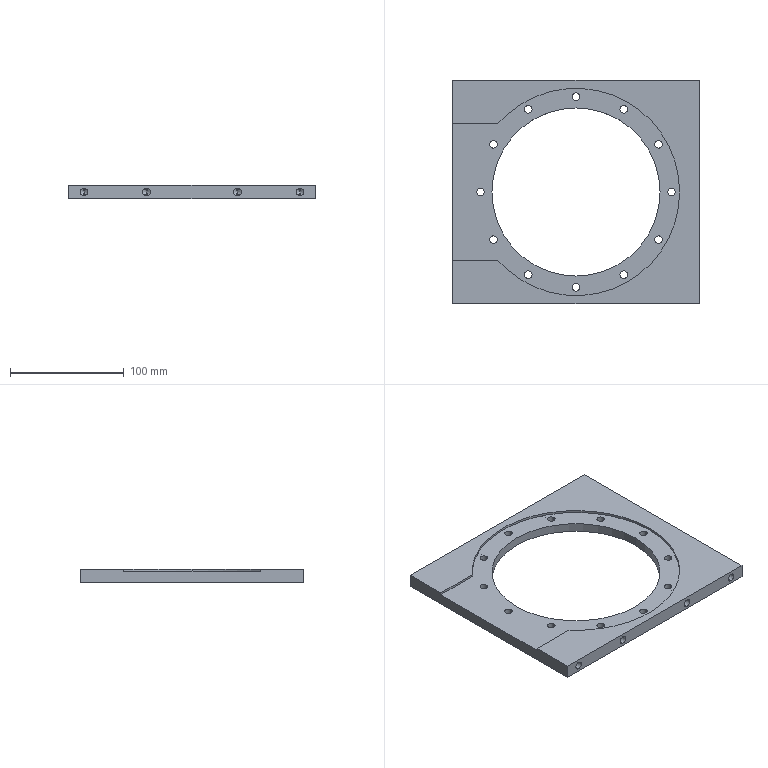Part | SolidWorks | features HoleWzd 3, ICE 2, Cut 1, Extrusion 1 | 1 solid | 72 faces | box 217 x 196.5 x 12 mm | volume 254363 mm3 | cylinder 46 | cone 16 | plane 10 | commonest cylinder face diameters 6.6 x24 6.8 x16 182.5 x4 148 x2